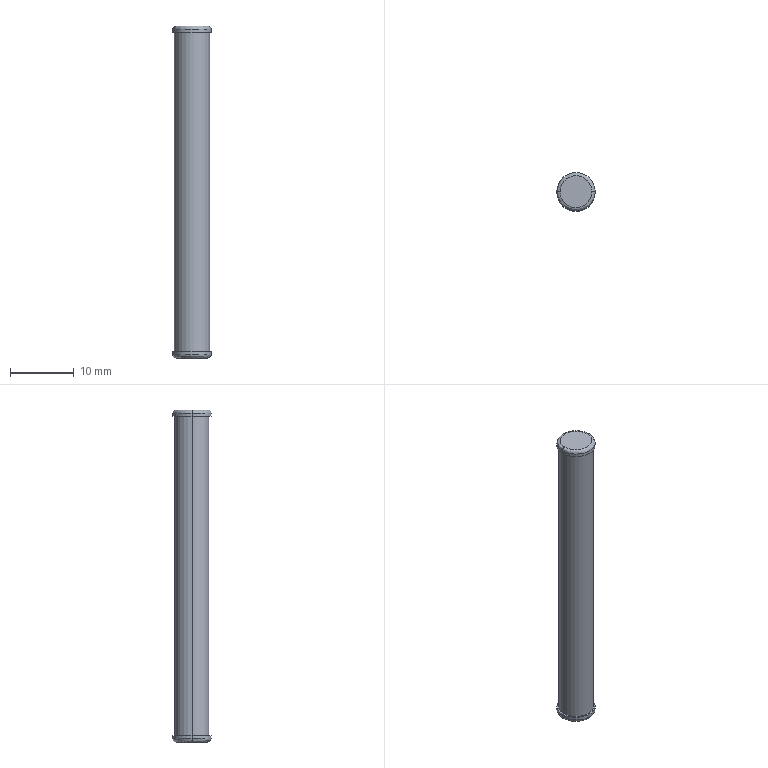Part | STEP file | 750038562 | 1 solid | 14 faces | box 6 x 6 x 52 mm | volume 1243 mm3 | cylinder 6 | spline 4 | plane 4 | commonest cylinder face diameters 6 x4 5.5 x2
STEP:
#1=CARTESIAN_POINT('',(-2.5,0.,-26.));
#2=VERTEX_POINT('',#1);
#3=CARTESIAN_POINT('',(2.5,0.,-26.));
#4=VERTEX_POINT('',#3);
#5=CARTESIAN_POINT('',(-2.5,0.,-26.));
#6=CARTESIAN_POINT('',(-2.5,-5.,-26.));
#7=CARTESIAN_POINT('',(2.5,-5.,-26.));
#8=CARTESIAN_POINT('',(2.5,0.,-26.));
#9=(BOUNDED_CURVE()B_SPLINE_CURVE(3,(#5,#6,#7,#8),.UNSPECIFIED.,.F.,.F.)B_SPLINE_CURVE_WITH_KNOTS((4,4),(0.,0.5),.UNSPECIFIED.)CURVE()GEOMETRIC_REPRESENTATION_ITEM()RATIONAL_B_SPLINE_CURVE((1.,0.3333,0.3333,1.))REPRESENTATION_ITEM(''));
#10=EDGE_CURVE('',#2,#4,#9,.T.);
#11=ORIENTED_EDGE('',*,*,#10,.T.);
#12=CARTESIAN_POINT('',(3.,0.,-25.5));
#13=VERTEX_POINT('',#12);
#14=CARTESIAN_POINT('',(2.5,0.,-25.5));
#15=DIRECTION('',(0.,-1.,0.));
#16=DIRECTION('',(1.,0.,0.));
#17=AXIS2_PLACEMENT_3D('',#14,#15,#16);
#18=CIRCLE('',#17,0.5);
#19=EDGE_CURVE('',#4,#13,#18,.T.);
#20=ORIENTED_EDGE('',*,*,#19,.T.);
#21=CARTESIAN_POINT('',(-3.,0.,-25.5));
#22=VERTEX_POINT('',#21);
#23=CARTESIAN_POINT('',(0.,0.,-25.5));
#24=DIRECTION('',(0.,0.,1.));
#25=DIRECTION('',(-1.,0.,0.));
#26=AXIS2_PLACEMENT_3D('',#23,#24,#25);
#27=CIRCLE('',#26,3.);
#28=EDGE_CURVE('',#22,#13,#27,.T.);
#29=ORIENTED_EDGE('',*,*,#28,.F.);
#30=CARTESIAN_POINT('',(-2.5,0.,-25.5));
#31=DIRECTION('',(0.,1.,0.));
#32=DIRECTION('',(-1.,0.,0.));
#33=AXIS2_PLACEMENT_3D('',#30,#31,#32);
#34=CIRCLE('',#33,0.5);
#35=EDGE_CURVE('',#2,#22,#34,.T.);
#36=ORIENTED_EDGE('',*,*,#35,.F.);
#37=EDGE_LOOP('',(#11,#20,#29,#36));
#38=FACE_OUTER_BOUND('',#37,.T.);
#39=CARTESIAN_POINT('',(2.5,0.,-26.));
#40=CARTESIAN_POINT('',(2.5,-5.,-26.));
#41=CARTESIAN_POINT('',(-2.5,-5.,-26.));
#42=CARTESIAN_POINT('',(-2.5,0.,-26.));
#43=CARTESIAN_POINT('',(2.793,0.,-26.));
#44=CARTESIAN_POINT('',(2.793,-5.586,-26.));
#45=CARTESIAN_POINT('',(-2.793,-5.586,-26.));
#46=CARTESIAN_POINT('',(-2.793,0.,-26.));
#47=CARTESIAN_POINT('',(3.,0.,-25.793));
#48=CARTESIAN_POINT('',(3.,-6.,-25.793));
#49=CARTESIAN_POINT('',(-3.,-6.,-25.793));
#50=CARTESIAN_POINT('',(-3.,0.,-25.793));
#51=CARTESIAN_POINT('',(3.,0.,-25.5));
#52=CARTESIAN_POINT('',(3.,-6.,-25.5));
#53=CARTESIAN_POINT('',(-3.,-6.,-25.5));
#54=CARTESIAN_POINT('',(-3.,0.,-25.5));
#55=(BOUNDED_SURFACE()B_SPLINE_SURFACE(3,3,((#39,#40,#41,#42),(#43,#44,#45,#46),(#47,#48,#49,#50),(#51,#52,#53,#54)),.UNSPECIFIED.,.F.,.F.,.T.)B_SPLINE_SURFACE_WITH_KNOTS((4,4),(4,4),(0.,1.),(0.,1.),.UNSPECIFIED.)GEOMETRIC_REPRESENTATION_ITEM()RATIONAL_B_SPLINE_SURFACE(((1.,0.3333,0.3333,1.),(0.8047,0.2682,0.2682,0.8047),(0.8047,0.2682,0.2682,0.8047),(1.,0.3333,0.3333,1.)))REPRESENTATION_ITEM('')SURFACE());
#56=ADVANCED_FACE('',(#38),#55,.T.);
#57=CARTESIAN_POINT('',(2.5,0.,26.));
#58=VERTEX_POINT('',#57);
#59=CARTESIAN_POINT('',(-2.5,0.,26.));
#60=VERTEX_POINT('',#59);
#61=CARTESIAN_POINT('',(2.5,0.,26.));
#62=CARTESIAN_POINT('',(2.5,-5.,26.));
#63=CARTESIAN_POINT('',(-2.5,-5.,26.));
#64=CARTESIAN_POINT('',(-2.5,0.,26.));
#65=(BOUNDED_CURVE()B_SPLINE_CURVE(3,(#61,#62,#63,#64),.UNSPECIFIED.,.F.,.T.)B_SPLINE_CURVE_WITH_KNOTS((4,4),(0.,0.5),.UNSPECIFIED.)CURVE()GEOMETRIC_REPRESENTATION_ITEM()RATIONAL_B_SPLINE_CURVE((1.,0.3333,0.3333,1.))REPRESENTATION_ITEM(''));
#66=EDGE_CURVE('',#58,#60,#65,.T.);
#67=ORIENTED_EDGE('',*,*,#66,.T.);
#68=CARTESIAN_POINT('',(-3.,0.,25.5));
#69=VERTEX_POINT('',#68);
#70=CARTESIAN_POINT('',(-2.5,0.,25.5));
#71=DIRECTION('',(0.,-1.,0.));
#72=DIRECTION('',(-1.,0.,0.));
#73=AXIS2_PLACEMENT_3D('',#70,#71,#72);
#74=CIRCLE('',#73,0.5);
#75=EDGE_CURVE('',#60,#69,#74,.T.);
#76=ORIENTED_EDGE('',*,*,#75,.T.);
#77=CARTESIAN_POINT('',(3.,0.,25.5));
#78=VERTEX_POINT('',#77);
#79=CARTESIAN_POINT('',(0.,0.,25.5));
#80=DIRECTION('',(0.,0.,-1.));
#81=DIRECTION('',(1.,0.,0.));
#82=AXIS2_PLACEMENT_3D('',#79,#80,#81);
#83=CIRCLE('',#82,3.);
#84=EDGE_CURVE('',#78,#69,#83,.T.);
#85=ORIENTED_EDGE('',*,*,#84,.F.);
#86=CARTESIAN_POINT('',(2.5,0.,25.5));
#87=DIRECTION('',(0.,1.,0.));
#88=DIRECTION('',(1.,0.,0.));
#89=AXIS2_PLACEMENT_3D('',#86,#87,#88);
#90=CIRCLE('',#89,0.5);
#91=EDGE_CURVE('',#58,#78,#90,.T.);
#92=ORIENTED_EDGE('',*,*,#91,.F.);
#93=EDGE_LOOP('',(#67,#76,#85,#92));
#94=FACE_OUTER_BOUND('',#93,.T.);
#95=CARTESIAN_POINT('',(-2.5,0.,26.));
#96=CARTESIAN_POINT('',(-2.5,-5.,26.));
#97=CARTESIAN_POINT('',(2.5,-5.,26.));
#98=CARTESIAN_POINT('',(2.5,0.,26.));
#99=CARTESIAN_POINT('',(-2.793,0.,26.));
#100=CARTESIAN_POINT('',(-2.793,-5.586,26.));
#101=CARTESIAN_POINT('',(2.793,-5.586,26.));
#102=CARTESIAN_POINT('',(2.793,0.,26.));
#103=CARTESIAN_POINT('',(-3.,0.,25.793));
#104=CARTESIAN_POINT('',(-3.,-6.,25.793));
#105=CARTESIAN_POINT('',(3.,-6.,25.793));
#106=CARTESIAN_POINT('',(3.,0.,25.793));
#107=CARTESIAN_POINT('',(-3.,0.,25.5));
#108=CARTESIAN_POINT('',(-3.,-6.,25.5));
#109=CARTESIAN_POINT('',(3.,-6.,25.5));
#110=CARTESIAN_POINT('',(3.,0.,25.5));
#111=(BOUNDED_SURFACE()B_SPLINE_SURFACE(3,3,((#95,#96,#97,#98),(#99,#100,#101,#102),(#103,#104,#105,#106),(#107,#108,#109,#110)),.UNSPECIFIED.,.F.,.F.,.F.)B_SPLINE_SURFACE_WITH_KNOTS((4,4),(4,4),(0.,1.),(0.,1.),.UNSPECIFIED.)GEOMETRIC_REPRESENTATION_ITEM()RATIONAL_B_SPLINE_SURFACE(((1.,0.3333,0.3333,1.),(0.8047,0.2682,0.2682,0.8047),(0.8047,0.2682,0.2682,0.8047),(1.,0.3333,0.3333,1.)))REPRESENTATION_ITEM('')SURFACE());
#112=ADVANCED_FACE('',(#94),#111,.T.);
#113=CARTESIAN_POINT('',(-2.75,0.,25.));
#114=VERTEX_POINT('',#113);
#115=CARTESIAN_POINT('',(2.75,0.,25.));
#116=VERTEX_POINT('',#115);
#117=CARTESIAN_POINT('',(0.,0.,25.));
#118=DIRECTION('',(0.,0.,-1.));
#119=DIRECTION('',(-1.,0.,0.));
#120=AXIS2_PLACEMENT_3D('',#117,#118,#119);
#121=CIRCLE('',#120,2.75);
#122=EDGE_CURVE('',#114,#116,#121,.T.);
#123=ORIENTED_EDGE('',*,*,#122,.T.);
#124=CARTESIAN_POINT('',(2.75,0.,-25.));
#125=VERTEX_POINT('',#124);
#126=CARTESIAN_POINT('',(2.75,0.,25.));
#127=DIRECTION('',(0.,0.,-1.));
#128=VECTOR('',#127,1000.);
#129=LINE('',#126,#128);
#130=EDGE_CURVE('',#116,#125,#129,.T.);
#131=ORIENTED_EDGE('',*,*,#130,.T.);
#132=CARTESIAN_POINT('',(-2.75,0.,-25.));
#133=VERTEX_POINT('',#132);
#134=CARTESIAN_POINT('',(0.,0.,-25.));
#135=DIRECTION('',(0.,0.,1.));
#136=DIRECTION('',(-1.,0.,0.));
#137=AXIS2_PLACEMENT_3D('',#134,#135,#136);
#138=CIRCLE('',#137,2.75);
#139=EDGE_CURVE('',#125,#133,#138,.T.);
#140=ORIENTED_EDGE('',*,*,#139,.T.);
#141=CARTESIAN_POINT('',(-2.75,0.,25.));
#142=DIRECTION('',(0.,0.,-1.));
#143=VECTOR('',#142,1000.);
#144=LINE('',#141,#143);
#145=EDGE_CURVE('',#114,#133,#144,.T.);
#146=ORIENTED_EDGE('',*,*,#145,.F.);
#147=EDGE_LOOP('',(#123,#131,#140,#146));
#148=FACE_OUTER_BOUND('',#147,.T.);
#149=CARTESIAN_POINT('',(0.,0.,25.));
#150=DIRECTION('',(0.,0.,-1.));
#151=DIRECTION('',(-1.,0.,0.));
#152=AXIS2_PLACEMENT_3D('',#149,#150,#151);
#153=CYLINDRICAL_SURFACE('',#152,2.75);
#154=ADVANCED_FACE('',(#148),#153,.T.);
#155=CARTESIAN_POINT('',(3.,0.,-25.));
#156=VERTEX_POINT('',#155);
#157=CARTESIAN_POINT('',(-3.,0.,-25.));
#158=VERTEX_POINT('',#157);
#159=CARTESIAN_POINT('',(0.,0.,-25.));
#160=DIRECTION('',(0.,0.,1.));
#161=DIRECTION('',(-1.,0.,0.));
#162=AXIS2_PLACEMENT_3D('',#159,#160,#161);
#163=CIRCLE('',#162,3.);
#164=EDGE_CURVE('',#156,#158,#163,.T.);
#165=ORIENTED_EDGE('',*,*,#164,.F.);
#166=CARTESIAN_POINT('',(3.,0.,-25.));
#167=DIRECTION('',(0.,0.,-1.));
#168=VECTOR('',#167,1000.);
#169=LINE('',#166,#168);
#170=EDGE_CURVE('',#156,#13,#169,.T.);
#171=ORIENTED_EDGE('',*,*,#170,.T.);
#172=CARTESIAN_POINT('',(0.,0.,-25.5));
#173=DIRECTION('',(0.,0.,1.));
#174=DIRECTION('',(-1.,0.,0.));
#175=AXIS2_PLACEMENT_3D('',#172,#173,#174);
#176=CIRCLE('',#175,3.);
#177=EDGE_CURVE('',#13,#22,#176,.T.);
#178=ORIENTED_EDGE('',*,*,#177,.T.);
#179=CARTESIAN_POINT('',(-3.,0.,-25.));
#180=DIRECTION('',(0.,0.,-1.));
#181=VECTOR('',#180,1000.);
#182=LINE('',#179,#181);
#183=EDGE_CURVE('',#158,#22,#182,.T.);
#184=ORIENTED_EDGE('',*,*,#183,.F.);
#185=EDGE_LOOP('',(#165,#171,#178,#184));
#186=FACE_OUTER_BOUND('',#185,.T.);
#187=CARTESIAN_POINT('',(0.,0.,-25.));
#188=DIRECTION('',(0.,0.,-1.));
#189=DIRECTION('',(-1.,0.,0.));
#190=AXIS2_PLACEMENT_3D('',#187,#188,#189);
#191=CYLINDRICAL_SURFACE('',#190,3.);
#192=ADVANCED_FACE('',(#186),#191,.T.);
#193=CARTESIAN_POINT('',(-3.,0.,25.));
#194=VERTEX_POINT('',#193);
#195=CARTESIAN_POINT('',(3.,0.,25.));
#196=VERTEX_POINT('',#195);
#197=CARTESIAN_POINT('',(0.,0.,25.));
#198=DIRECTION('',(0.,0.,-1.));
#199=DIRECTION('',(1.,0.,0.));
#200=AXIS2_PLACEMENT_3D('',#197,#198,#199);
#201=CIRCLE('',#200,3.);
#202=EDGE_CURVE('',#194,#196,#201,.T.);
#203=ORIENTED_EDGE('',*,*,#202,.F.);
#204=CARTESIAN_POINT('',(-3.,0.,25.));
#205=DIRECTION('',(0.,0.,1.));
#206=VECTOR('',#205,1000.);
#207=LINE('',#204,#206);
#208=EDGE_CURVE('',#194,#69,#207,.T.);
#209=ORIENTED_EDGE('',*,*,#208,.T.);
#210=CARTESIAN_POINT('',(0.,0.,25.5));
#211=DIRECTION('',(0.,0.,-1.));
#212=DIRECTION('',(1.,0.,0.));
#213=AXIS2_PLACEMENT_3D('',#210,#211,#212);
#214=CIRCLE('',#213,3.);
#215=EDGE_CURVE('',#69,#78,#214,.T.);
#216=ORIENTED_EDGE('',*,*,#215,.T.);
#217=CARTESIAN_POINT('',(3.,0.,25.));
#218=DIRECTION('',(0.,0.,1.));
#219=VECTOR('',#218,1000.);
#220=LINE('',#217,#219);
#221=EDGE_CURVE('',#196,#78,#220,.T.);
#222=ORIENTED_EDGE('',*,*,#221,.F.);
#223=EDGE_LOOP('',(#203,#209,#216,#222));
#224=FACE_OUTER_BOUND('',#223,.T.);
#225=CARTESIAN_POINT('',(0.,0.,25.));
#226=DIRECTION('',(0.,0.,1.));
#227=DIRECTION('',(1.,0.,0.));
#228=AXIS2_PLACEMENT_3D('',#225,#226,#227);
#229=CYLINDRICAL_SURFACE('',#228,3.);
#230=ADVANCED_FACE('',(#224),#229,.T.);
#231=ORIENTED_EDGE('',*,*,#130,.F.);
#232=CARTESIAN_POINT('',(0.,0.,25.));
#233=DIRECTION('',(0.,0.,-1.));
#234=DIRECTION('',(-1.,0.,0.));
#235=AXIS2_PLACEMENT_3D('',#232,#233,#234);
#236=CIRCLE('',#235,2.75);
#237=EDGE_CURVE('',#116,#114,#236,.T.);
#238=ORIENTED_EDGE('',*,*,#237,.T.);
#239=ORIENTED_EDGE('',*,*,#145,.T.);
#240=CARTESIAN_POINT('',(0.,0.,-25.));
#241=DIRECTION('',(0.,0.,1.));
#242=DIRECTION('',(-1.,0.,0.));
#243=AXIS2_PLACEMENT_3D('',#240,#241,#242);
#244=CIRCLE('',#243,2.75);
#245=EDGE_CURVE('',#133,#125,#244,.T.);
#246=ORIENTED_EDGE('',*,*,#245,.T.);
#247=EDGE_LOOP('',(#231,#238,#239,#246));
#248=FACE_OUTER_BOUND('',#247,.T.);
#249=CARTESIAN_POINT('',(0.,0.,25.));
#250=DIRECTION('',(0.,0.,-1.));
#251=DIRECTION('',(-1.,0.,0.));
#252=AXIS2_PLACEMENT_3D('',#249,#250,#251);
#253=CYLINDRICAL_SURFACE('',#252,2.75);
#254=ADVANCED_FACE('',(#248),#253,.T.);
#255=ORIENTED_EDGE('',*,*,#245,.F.);
#256=ORIENTED_EDGE('',*,*,#139,.F.);
#257=EDGE_LOOP('',(#255,#256));
#258=FACE_BOUND('',#257,.T.);
#259=CARTESIAN_POINT('',(0.,0.,-25.));
#260=DIRECTION('',(0.,0.,1.));
#261=DIRECTION('',(-1.,0.,0.));
#262=AXIS2_PLACEMENT_3D('',#259,#260,#261);
#263=CIRCLE('',#262,3.);
#264=EDGE_CURVE('',#158,#156,#263,.T.);
#265=ORIENTED_EDGE('',*,*,#264,.T.);
#266=ORIENTED_EDGE('',*,*,#164,.T.);
#267=EDGE_LOOP('',(#265,#266));
#268=FACE_OUTER_BOUND('',#267,.T.);
#269=CARTESIAN_POINT('',(0.,0.,-25.));
#270=DIRECTION('',(0.,0.,1.));
#271=DIRECTION('',(1.,0.,0.));
#272=AXIS2_PLACEMENT_3D('',#269,#270,#271);
#273=PLANE('',#272);
#274=ADVANCED_FACE('',(#258,#268),#273,.T.);
#275=ORIENTED_EDGE('',*,*,#122,.F.);
#276=ORIENTED_EDGE('',*,*,#237,.F.);
#277=EDGE_LOOP('',(#275,#276));
#278=FACE_BOUND('',#277,.T.);
#279=CARTESIAN_POINT('',(0.,0.,25.));
#280=DIRECTION('',(0.,0.,-1.));
#281=DIRECTION('',(1.,0.,0.));
#282=AXIS2_PLACEMENT_3D('',#279,#280,#281);
#283=CIRCLE('',#282,3.);
#284=EDGE_CURVE('',#196,#194,#283,.T.);
#285=ORIENTED_EDGE('',*,*,#284,.T.);
#286=ORIENTED_EDGE('',*,*,#202,.T.);
#287=EDGE_LOOP('',(#285,#286));
#288=FACE_OUTER_BOUND('',#287,.T.);
#289=CARTESIAN_POINT('',(0.,0.,25.));
#290=DIRECTION('',(0.,0.,-1.));
#291=DIRECTION('',(-1.,0.,0.));
#292=AXIS2_PLACEMENT_3D('',#289,#290,#291);
#293=PLANE('',#292);
#294=ADVANCED_FACE('',(#278,#288),#293,.T.);
#295=ORIENTED_EDGE('',*,*,#170,.F.);
#296=ORIENTED_EDGE('',*,*,#264,.F.);
#297=ORIENTED_EDGE('',*,*,#183,.T.);
#298=ORIENTED_EDGE('',*,*,#28,.T.);
#299=EDGE_LOOP('',(#295,#296,#297,#298));
#300=FACE_OUTER_BOUND('',#299,.T.);
#301=CARTESIAN_POINT('',(0.,0.,-25.));
#302=DIRECTION('',(0.,0.,-1.));
#303=DIRECTION('',(-1.,0.,0.));
#304=AXIS2_PLACEMENT_3D('',#301,#302,#303);
#305=CYLINDRICAL_SURFACE('',#304,3.);
#306=ADVANCED_FACE('',(#300),#305,.T.);
#307=ORIENTED_EDGE('',*,*,#208,.F.);
#308=ORIENTED_EDGE('',*,*,#284,.F.);
#309=ORIENTED_EDGE('',*,*,#221,.T.);
#310=ORIENTED_EDGE('',*,*,#84,.T.);
#311=EDGE_LOOP('',(#307,#308,#309,#310));
#312=FACE_OUTER_BOUND('',#311,.T.);
#313=CARTESIAN_POINT('',(0.,0.,25.));
#314=DIRECTION('',(0.,0.,1.));
#315=DIRECTION('',(1.,0.,0.));
#316=AXIS2_PLACEMENT_3D('',#313,#314,#315);
#317=CYLINDRICAL_SURFACE('',#316,3.);
#318=ADVANCED_FACE('',(#312),#317,.T.);
#319=ORIENTED_EDGE('',*,*,#19,.F.);
#320=CARTESIAN_POINT('',(2.5,0.,-26.));
#321=CARTESIAN_POINT('',(2.5,5.,-26.));
#322=CARTESIAN_POINT('',(-2.5,5.,-26.));
#323=CARTESIAN_POINT('',(-2.5,0.,-26.));
#324=(BOUNDED_CURVE()B_SPLINE_CURVE(3,(#320,#321,#322,#323),.UNSPECIFIED.,.F.,.F.)B_SPLINE_CURVE_WITH_KNOTS((4,4),(0.5,1.),.UNSPECIFIED.)CURVE()GEOMETRIC_REPRESENTATION_ITEM()RATIONAL_B_SPLINE_CURVE((1.,0.3333,0.3333,1.))REPRESENTATION_ITEM(''));
#325=EDGE_CURVE('',#4,#2,#324,.T.);
#326=ORIENTED_EDGE('',*,*,#325,.T.);
#327=ORIENTED_EDGE('',*,*,#35,.T.);
#328=ORIENTED_EDGE('',*,*,#177,.F.);
#329=EDGE_LOOP('',(#319,#326,#327,#328));
#330=FACE_OUTER_BOUND('',#329,.T.);
#331=CARTESIAN_POINT('',(-2.5,0.,-26.));
#332=CARTESIAN_POINT('',(-2.5,5.,-26.));
#333=CARTESIAN_POINT('',(2.5,5.,-26.));
#334=CARTESIAN_POINT('',(2.5,0.,-26.));
#335=CARTESIAN_POINT('',(-2.793,0.,-26.));
#336=CARTESIAN_POINT('',(-2.793,5.586,-26.));
#337=CARTESIAN_POINT('',(2.793,5.586,-26.));
#338=CARTESIAN_POINT('',(2.793,0.,-26.));
#339=CARTESIAN_POINT('',(-3.,0.,-25.793));
#340=CARTESIAN_POINT('',(-3.,6.,-25.793));
#341=CARTESIAN_POINT('',(3.,6.,-25.793));
#342=CARTESIAN_POINT('',(3.,0.,-25.793));
#343=CARTESIAN_POINT('',(-3.,0.,-25.5));
#344=CARTESIAN_POINT('',(-3.,6.,-25.5));
#345=CARTESIAN_POINT('',(3.,6.,-25.5));
#346=CARTESIAN_POINT('',(3.,0.,-25.5));
#347=(BOUNDED_SURFACE()B_SPLINE_SURFACE(3,3,((#331,#332,#333,#334),(#335,#336,#337,#338),(#339,#340,#341,#342),(#343,#344,#345,#346)),.UNSPECIFIED.,.F.,.F.,.T.)B_SPLINE_SURFACE_WITH_KNOTS((4,4),(4,4),(0.,1.),(0.,1.),.UNSPECIFIED.)GEOMETRIC_REPRESENTATION_ITEM()RATIONAL_B_SPLINE_SURFACE(((1.,0.3333,0.3333,1.),(0.8047,0.2682,0.2682,0.8047),(0.8047,0.2682,0.2682,0.8047),(1.,0.3333,0.3333,1.)))REPRESENTATION_ITEM('')SURFACE());
#348=ADVANCED_FACE('',(#330),#347,.T.);
#349=ORIENTED_EDGE('',*,*,#75,.F.);
#350=CARTESIAN_POINT('',(-2.5,0.,26.));
#351=CARTESIAN_POINT('',(-2.5,5.,26.));
#352=CARTESIAN_POINT('',(2.5,5.,26.));
#353=CARTESIAN_POINT('',(2.5,0.,26.));
#354=(BOUNDED_CURVE()B_SPLINE_CURVE(3,(#350,#351,#352,#353),.UNSPECIFIED.,.F.,.T.)B_SPLINE_CURVE_WITH_KNOTS((4,4),(0.5,1.),.UNSPECIFIED.)CURVE()GEOMETRIC_REPRESENTATION_ITEM()RATIONAL_B_SPLINE_CURVE((1.,0.3333,0.3333,1.))REPRESENTATION_ITEM(''));
#355=EDGE_CURVE('',#60,#58,#354,.T.);
#356=ORIENTED_EDGE('',*,*,#355,.T.);
#357=ORIENTED_EDGE('',*,*,#91,.T.);
#358=ORIENTED_EDGE('',*,*,#215,.F.);
#359=EDGE_LOOP('',(#349,#356,#357,#358));
#360=FACE_OUTER_BOUND('',#359,.T.);
#361=CARTESIAN_POINT('',(2.5,0.,26.));
#362=CARTESIAN_POINT('',(2.5,5.,26.));
#363=CARTESIAN_POINT('',(-2.5,5.,26.));
#364=CARTESIAN_POINT('',(-2.5,0.,26.));
#365=CARTESIAN_POINT('',(2.793,0.,26.));
#366=CARTESIAN_POINT('',(2.793,5.586,26.));
#367=CARTESIAN_POINT('',(-2.793,5.586,26.));
#368=CARTESIAN_POINT('',(-2.793,0.,26.));
#369=CARTESIAN_POINT('',(3.,0.,25.793));
#370=CARTESIAN_POINT('',(3.,6.,25.793));
#371=CARTESIAN_POINT('',(-3.,6.,25.793));
#372=CARTESIAN_POINT('',(-3.,0.,25.793));
#373=CARTESIAN_POINT('',(3.,0.,25.5));
#374=CARTESIAN_POINT('',(3.,6.,25.5));
#375=CARTESIAN_POINT('',(-3.,6.,25.5));
#376=CARTESIAN_POINT('',(-3.,0.,25.5));
#377=(BOUNDED_SURFACE()B_SPLINE_SURFACE(3,3,((#361,#362,#363,#364),(#365,#366,#367,#368),(#369,#370,#371,#372),(#373,#374,#375,#376)),.UNSPECIFIED.,.F.,.F.,.F.)B_SPLINE_SURFACE_WITH_KNOTS((4,4),(4,4),(0.,1.),(0.,1.),.UNSPECIFIED.)GEOMETRIC_REPRESENTATION_ITEM()RATIONAL_B_SPLINE_SURFACE(((1.,0.3333,0.3333,1.),(0.8047,0.2682,0.2682,0.8047),(0.8047,0.2682,0.2682,0.8047),(1.,0.3333,0.3333,1.)))REPRESENTATION_ITEM('')SURFACE());
#378=ADVANCED_FACE('',(#360),#377,.T.);
#379=ORIENTED_EDGE('',*,*,#10,.F.);
#380=ORIENTED_EDGE('',*,*,#325,.F.);
#381=EDGE_LOOP('',(#379,#380));
#382=FACE_OUTER_BOUND('',#381,.T.);
#383=CARTESIAN_POINT('',(0.,0.,-26.));
#384=DIRECTION('',(0.,0.,-1.));
#385=DIRECTION('',(-1.,0.,0.));
#386=AXIS2_PLACEMENT_3D('',#383,#384,#385);
#387=PLANE('',#386);
#388=ADVANCED_FACE('',(#382),#387,.T.);
#389=ORIENTED_EDGE('',*,*,#66,.F.);
#390=ORIENTED_EDGE('',*,*,#355,.F.);
#391=EDGE_LOOP('',(#389,#390));
#392=FACE_OUTER_BOUND('',#391,.T.);
#393=CARTESIAN_POINT('',(0.,0.,26.));
#394=DIRECTION('',(0.,0.,1.));
#395=DIRECTION('',(1.,0.,0.));
#396=AXIS2_PLACEMENT_3D('',#393,#394,#395);
#397=PLANE('',#396);
#398=ADVANCED_FACE('',(#392),#397,.T.);
#399=CLOSED_SHELL('',(#56,#112,#154,#192,#230,#254,#274,#294,#306,#318,#348,#378,#388,#398));
#400=MANIFOLD_SOLID_BREP('',#399);
#401=CARTESIAN_POINT('',(0.,0.,0.));
#402=DIRECTION('',(0.,0.,1.));
#403=DIRECTION('',(1.,0.,0.));
#404=AXIS2_PLACEMENT_3D('',#401,#402,#403);
#405=(LENGTH_UNIT()NAMED_UNIT(*)SI_UNIT(.MILLI.,.METRE.));
#406=UNCERTAINTY_MEASURE_WITH_UNIT(LENGTH_MEASURE(0.00001),#405,'','');
#407=(NAMED_UNIT(*)PLANE_ANGLE_UNIT()SI_UNIT($,.RADIAN.));
#408=(NAMED_UNIT(*)SI_UNIT($,.STERADIAN.)SOLID_ANGLE_UNIT());
#409=(GEOMETRIC_REPRESENTATION_CONTEXT(3)GLOBAL_UNCERTAINTY_ASSIGNED_CONTEXT((#406))GLOBAL_UNIT_ASSIGNED_CONTEXT((#405,#407,#408))REPRESENTATION_CONTEXT('',''));
#410=ADVANCED_BREP_SHAPE_REPRESENTATION('',(#400,#404),#409);